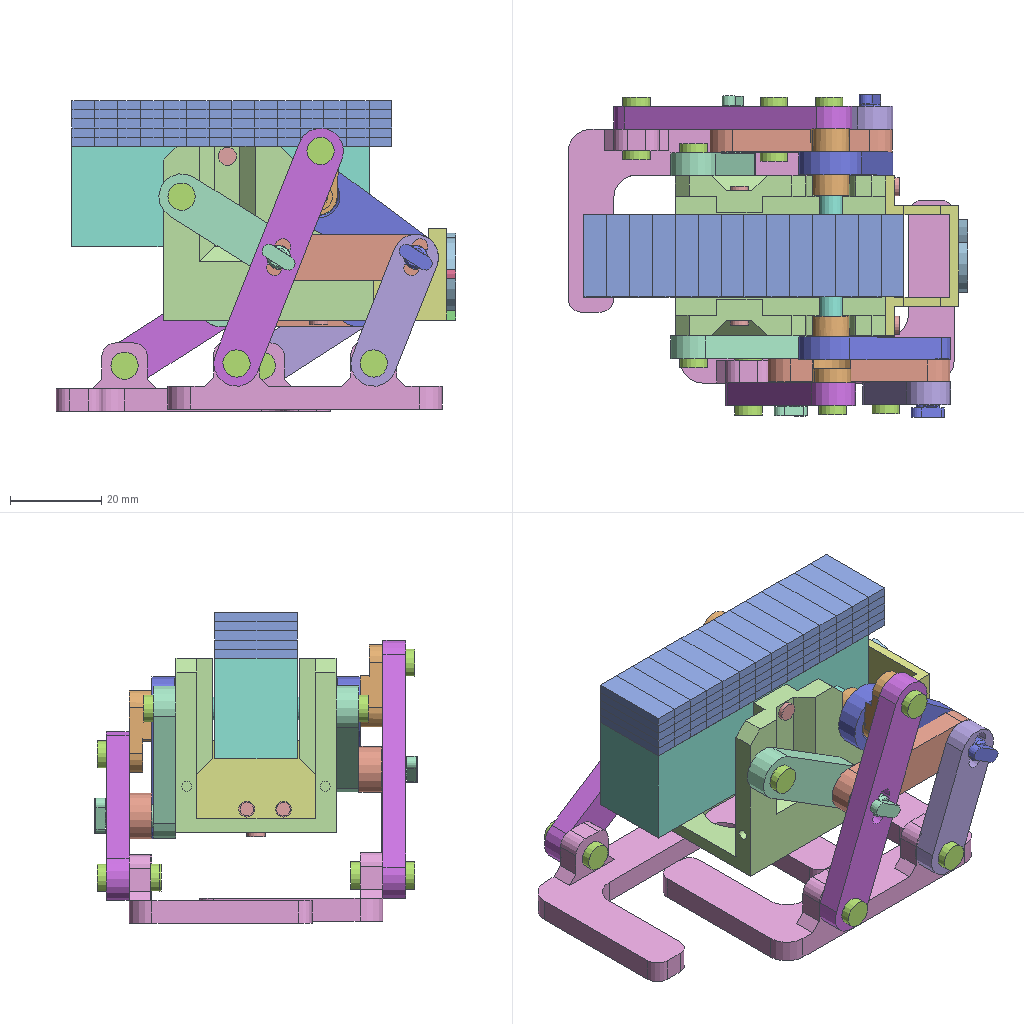Assembly | NX | 13 different items | 112 placed | box 87 x 71 x 68 mm
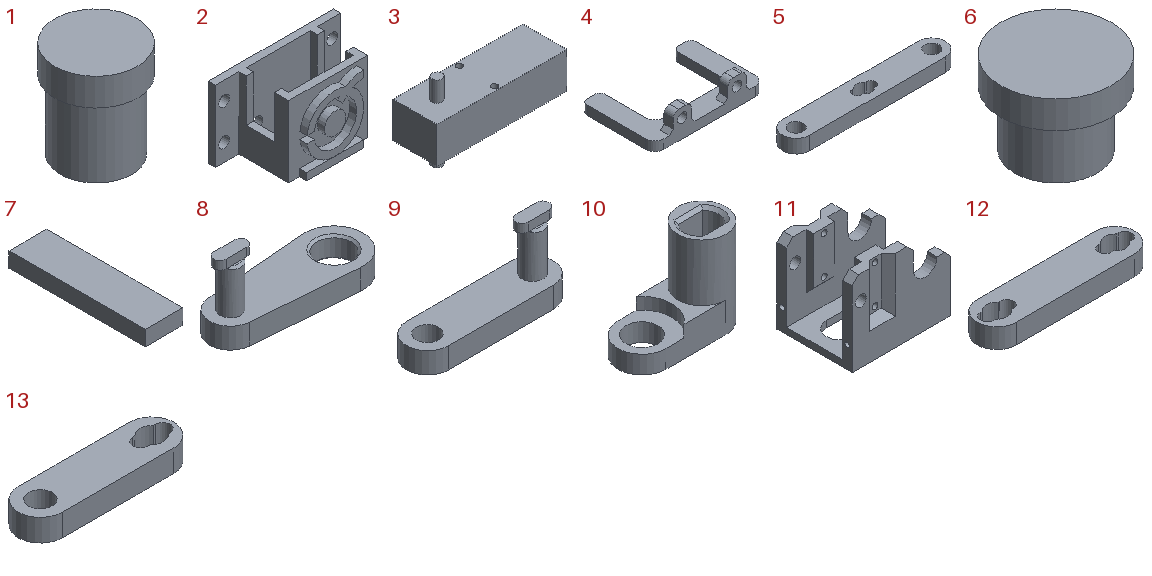Parts list (item | quantity | size | volume | features):
1 | x12 | 6 x 6 x 7 mm | 162.734 mm3 | features CYLINDER 2, DATUM_CSYS 1
2 | x1 | 35 x 18 x 20 mm | 3071 mm3 | features BREP 4
3 | x1 | 65 x 22 x 38 mm | 25878 mm3 | features BREP 1
4 | x2 | 60 x 40 x 15 mm | 6735 mm3 | features BREP 1
5 | x2 | 60 x 10 x 5 mm | 2515 mm3 | features BREP 1
6 | x13 | 4 x 4 x 3 mm | 26.704 mm3 | features CYLINDER 2, DATUM_CSYS 1
7 | x70 | 5 x 18 x 2 mm | 180 mm3 | features DATUM_CSYS 2, EXTRUDE 1, SKETCH 1
8 | x2 | 37 x 14 x 17.5 mm | 2058 mm3 | features BREP 1
9 | x2 | 35 x 10 x 17.5 mm | 1782 mm3 | features BREP 1
10 | x2 | 18 x 8 x 14.5 mm | 713.021 mm3 | features BREP 1
11 | x1 | 46 x 35 x 38 mm | 15547 mm3 | features BREP 1
12 | x2 | 40 x 10 x 5 mm | 1578 mm3 | features BREP 1
13 | x2 | 35 x 10 x 5 mm | 1375 mm3 | features BREP 1
Mates (type | each side: item.copy, entity, surface, feature):
Concentric | 1.1 edge | 13.1 edge | 2 times
Concentric | 1.1 edge | 5.1 edge | 4 times
Concentric | 1.1 edge | 9.1 edge | 2 times
Concentric | 6.1 edge | 2.1 edge | 6 times
Concentric | 1.1 edge | 4.1 edge | 4 times
Touch | 7.1 face plane Extrude(1) | 3.1 face plane Body(1) | 3 times
Concentric | 6.1 edge | 10.1 edge | 2 times
Concentric | 6.1 edge | 11.1 edge | 5 times